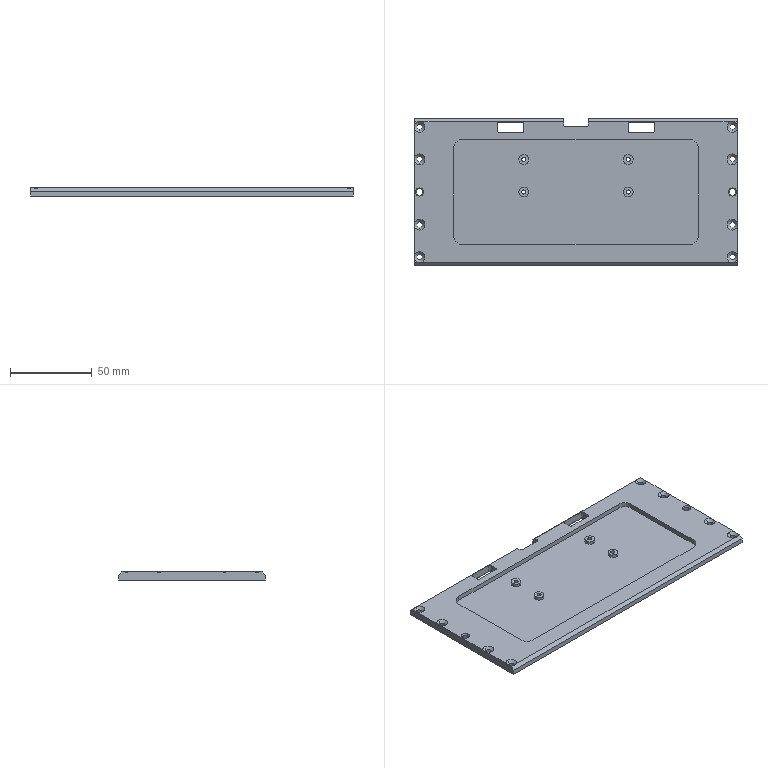NC program | NX | posted with a generic post | part box 198 x 90 x 5 mm
Lines 3800 to 4593 of 7766:
(ZLEVEL_PROFILE_COPY_1_COPY_COPY_COPY_1 , TOOL : D6A45)
N7532 T01 M6
N7534 G54
N7536 G17 G0 G90 X-98.549 Y18.596 S9500 M3
N7538 G43 Z30. H1
N7540 Z1.5
N7542 G94 G1 X-98.417 Y18.395 Z1.487 F1000.
N7544 X-98.284 Y18.195 Z1.475
N7546 X-97.848 Y17.753 Z1.442
N7548 X-97.329 Y17.413 Z1.41
N7550 X-96.75 Y17.192 Z1.377
N7552 X-96.137 Y17.098 Z1.345
N7554 X-95.518 Y17.136 Z1.312
N7556 X-94.921 Y17.304 Z1.28
N7558 X-94.373 Y17.596 Z1.247
N7560 X-93.998 Y17.898 Z1.222
N7562 X-93.598 Y18.372 Z1.189
N7564 X-93.306 Y18.92 Z1.157
N7566 X-93.138 Y19.517 Z1.124
N7568 X-93.1 Y20.136 Z1.092
N7570 X-93.194 Y20.749 Z1.059
N7572 X-93.416 Y21.328 Z1.027
N7574 X-93.756 Y21.847 Z0.994
N7576 X-93.923 Y22.02 Z0.982
N7578 X-94.092 Y22.193 Z0.969
N7580 X-94.624 Y22.56 Z0.935
N7582 X-95.224 Y22.801 Z0.901
N7584 X-95.862 Y22.903 Z0.868
N7586 X-96.507 Y22.862 Z0.834
N7588 X-97.128 Y22.681 Z0.8
N7590 X-97.692 Y22.366 Z0.766
N7592 X-98.174 Y21.936 Z0.732
N7594 X-98.32 Y21.743 Z0.719
N7596 X-98.46 Y21.586 Z0.708
N7598 X-98.679 Y21.219 Z0.686
N7600 X-98.835 Y20.79 Z0.662
N7602 X-98.933 Y20.214 Z0.631
N7604 X-98.917 Y19.63 Z0.601
N7606 X-98.79 Y19.06 Z0.57
N7608 X-98.694 Y18.834 Z0.557
N7610 X-98.679 Y18.795 Z0.555
N7612 X-98.417 Y18.395 Z0.53
N7614 X-98.284 Y18.195 Z0.517
N7616 X-97.848 Y17.753 Z0.485
N7618 X-97.329 Y17.413 Z0.452
N7620 X-96.75 Y17.192 Z0.42
N7622 X-96.137 Y17.098 Z0.387
N7624 X-95.518 Y17.136 Z0.355
N7626 X-94.921 Y17.304 Z0.322
N7628 X-94.373 Y17.596 Z0.29
N7630 X-93.998 Y17.898 Z0.265
N7632 X-93.598 Y18.372 Z0.232
N7634 X-93.306 Y18.92 Z0.2
N7636 X-93.138 Y19.517 Z0.167
N7638 X-93.1 Y20.136 Z0.135
N7640 X-93.194 Y20.749 Z0.102
N7642 X-93.416 Y21.328 Z0.07
N7644 X-93.756 Y21.847 Z0.037
N7646 X-93.923 Y22.02 Z0.024
N7648 X-94.092 Y22.193 Z0.012
N7650 X-94.624 Y22.56 Z-0.022
N7652 X-95.224 Y22.801 Z-0.056
N7654 X-95.862 Y22.903 Z-0.09
N7656 X-96.507 Y22.862 Z-0.124
N7658 X-97.128 Y22.681 Z-0.158
N7660 X-97.692 Y22.366 Z-0.191
N7662 X-98.174 Y21.936 Z-0.225
N7664 X-98.32 Y21.743 Z-0.238
N7666 X-98.46 Y21.586 Z-0.249
N7668 X-98.679 Y21.219 Z-0.271
N7670 X-98.835 Y20.79 Z-0.295
N7672 X-98.933 Y20.214 Z-0.326
N7674 X-98.917 Y19.63 Z-0.357
N7676 X-98.79 Y19.06 Z-0.387
N7678 X-98.694 Y18.834 Z-0.4
N7680 X-98.679 Y18.795 F1300.
N7682 X-98.417 Y18.395
N7684 G3 X-93.923 Y22.02 R-2.899
N7686 X-98.32 Y21.743 R2.904
N7688 X-98.751 Y21.02 R2.219
N7690 X-98.694 Y18.834 R3.
N7692 G1 X-98.678 Y18.795 Z-0.401
N7694 X-98.543 Y18.599 Z-0.407
N7696 X-98.381 Y18.366 Z-0.413
N7698 X-98.246 Y18.197 Z-0.418
N7700 X-98.099 Y18.037 Z-0.424
N7702 X-97.925 Y17.874 Z-0.429
N7704 X-97.739 Y17.726 Z-0.435
N7706 X-97.54 Y17.597 Z-0.44
N7708 X-97.334 Y17.479 Z-0.446
N7710 X-97.116 Y17.387 Z-0.452
N7712 X-96.894 Y17.304 Z-0.457
N7714 X-96.665 Y17.251 Z-0.463
N7716 X-96.435 Y17.203 Z-0.468
N7718 X-96.195 Y17.184 Z-0.474
N7720 X-95.966 Y17.182 Z-0.479
N7722 X-95.733 Y17.206 Z-0.485
N7724 X-95.502 Y17.24 Z-0.49
N7726 X-95.277 Y17.298 Z-0.496
N7728 X-95.056 Y17.372 Z-0.501
N7730 X-94.843 Y17.463 Z-0.507
N7732 X-94.739 Y17.516 Z-0.51
N7734 X-94.639 Y17.575 Z-0.512
N7736 X-94.443 Y17.697 Z-0.518
N7738 X-94.263 Y17.843 Z-0.523
N7740 X-94.165 Y17.926 Z-0.526
N7742 X-94.048 Y18.044 Z-0.53
N7744 X-93.938 Y18.168 Z-0.534
N7746 X-93.796 Y18.348 Z-0.539
N7748 X-93.67 Y18.54 Z-0.545
N7750 X-93.564 Y18.742 Z-0.55
N7752 X-93.469 Y18.95 Z-0.556
N7754 X-93.4 Y19.167 Z-0.561
N7756 X-93.337 Y19.386 Z-0.566
N7758 X-93.303 Y19.613 Z-0.572
N7760 X-93.285 Y19.836 Z-0.577
N7762 X-93.291 Y20.062 Z-0.582
N7764 X-93.309 Y20.287 Z-0.588
N7766 X-93.348 Y20.508 Z-0.593
N7768 X-93.403 Y20.726 Z-0.598
N7770 X-93.477 Y20.937 Z-0.604
N7772 X-93.568 Y21.142 Z-0.609
N7774 X-93.674 Y21.338 Z-0.614
N7776 X-93.799 Y21.524 Z-0.62
N7778 X-93.937 Y21.697 Z-0.625
N7780 X-94.088 Y21.86 Z-0.63
N7782 X-94.163 Y21.929 Z-0.632
N7784 X-94.239 Y21.997 Z-0.635
N7786 X-94.408 Y22.129 Z-0.64
N7788 X-94.585 Y22.239 Z-0.645
N7790 X-94.765 Y22.343 Z-0.65
N7792 X-94.956 Y22.423 Z-0.655
N7794 X-95.149 Y22.498 Z-0.66
N7796 X-95.35 Y22.546 Z-0.664
N7798 X-95.552 Y22.592 Z-0.669
N7800 X-95.962 Y22.621 Z-0.679
N7802 X-96.371 Y22.585 Z-0.689
N7804 X-96.768 Y22.487 Z-0.698
N7806 X-96.957 Y22.41 Z-0.703
N7808 X-97.143 Y22.329 Z-0.708
N7810 X-97.487 Y22.114 Z-0.718
N7812 X-97.791 Y21.848 Z-0.727
N7814 X-98.052 Y21.542 Z-0.737
N7816 X-98.109 Y21.46 Z-0.739
N7818 X-98.202 Y21.323 Z-0.743
N7820 X-98.327 Y21.114 Z-0.749
N7822 X-98.38 Y21.004 Z-0.752
N7824 X-98.42 Y20.889 Z-0.754
N7826 X-98.469 Y20.703 Z-0.759
N7828 X-98.516 Y20.515 Z-0.764
N7830 X-98.537 Y20.325 Z-0.768
N7832 X-98.556 Y20.133 Z-0.773
N7834 Y20.015 Z-0.775
N7836 X-98.535 Y19.734 Z-0.782
N7838 X-98.498 Y19.547 Z-0.787
N7840 X-98.46 Y19.361 Z-0.791
N7842 X-98.4 Y19.182 Z-0.796
N7844 X-98.325 Y19.009 Z-0.8
N7846 X-98.266 Y18.899 Z-0.803
N7848 X-98.199 Y18.793 Z-0.807
N7850 X-98.051 Y18.594 Z-0.814
N7852 X-97.917 Y18.432 Z-0.82
N7854 X-97.775 Y18.279 Z-0.825
N7856 X-97.616 Y18.143 Z-0.831
N7858 X-97.452 Y18.014 Z-0.837
N7860 X-97.36 Y17.954 Z-0.84
N7862 X-97.091 Y17.808 Z-0.848
N7864 X-96.879 Y17.722 Z-0.855
N7866 X-96.703 Y17.666 Z-0.86
N7868 X-96.501 Y17.626 Z-0.866
N7870 X-96.298 Y17.595 Z-0.871
N7872 X-96.152 Y17.584 Z-0.875
N7874 X-96.015 Y17.577 Z-0.879
N7876 X-95.888 Y17.591 Z-0.883
N7878 X-95.686 Y17.614 Z-0.888
N7880 X-95.486 Y17.655 Z-0.894
N7882 X-95.29 Y17.709 Z-0.9
N7884 X-95.102 Y17.786 Z-0.905
N7886 X-94.921 Y17.875 Z-0.911
N7888 X-94.747 Y17.979 Z-0.917
N7890 X-94.585 Y18.098 Z-0.922
N7892 X-94.431 Y18.227 Z-0.928
N7894 X-94.294 Y18.373 Z-0.933
N7896 X-94.161 Y18.522 Z-0.939
N7898 X-94.091 Y18.625 Z-0.942
N7900 X-94.019 Y18.742 Z-0.946
N7902 X-93.949 Y18.86 Z-0.95
N7904 X-93.869 Y19.042 Z-0.955
N7906 X-93.797 Y19.227 Z-0.961
N7908 X-93.747 Y19.417 Z-0.966
N7910 X-93.708 Y19.611 Z-0.972
N7912 X-93.689 Y19.806 Z-0.977
N7914 X-93.686 Y20.003 Z-0.983
N7916 X-93.701 Y20.198 Z-0.988
N7918 X-93.73 Y20.392 Z-0.994
N7920 X-93.78 Y20.579 Z-0.999
N7922 X-93.838 Y20.765 Z-1.004
N7924 X-93.922 Y20.952 Z-1.01
N7926 X-94.007 Y21.114 Z-1.015
N7928 X-94.231 Y21.427 Z-1.026
N7930 X-94.367 Y21.562 Z-1.031
N7932 X-94.503 Y21.697 Z-1.037
N7934 X-94.605 Y21.775 Z-1.04
N7936 X-94.71 Y21.846 Z-1.044
N7938 X-94.817 Y21.915 Z-1.047
N7940 X-94.986 Y22. Z-1.052
N7942 X-95.16 Y22.076 Z-1.058
N7944 X-95.34 Y22.134 Z-1.063
N7946 X-95.524 Y22.178 Z-1.068
N7948 X-95.71 Y22.202 Z-1.073
N7950 X-95.897 Y22.217 Z-1.079
N7952 X-96.104 Y22.21 Z-1.084
N7954 X-96.27 Y22.194 Z-1.089
N7956 X-96.632 Y22.107 Z-1.099
N7958 X-96.804 Y22.039 Z-1.105
N7960 X-96.973 Y21.961 Z-1.11
N7962 X-97.128 Y21.862 Z-1.115
N7964 X-97.282 Y21.761 Z-1.12
N7966 X-97.419 Y21.639 Z-1.125
N7968 X-97.552 Y21.512 Z-1.13
N7970 X-97.644 Y21.406 Z-1.134
N7972 X-97.72 Y21.312 Z-1.137
N7974 X-97.789 Y21.214 Z-1.141
N7976 X-97.887 Y21.062 Z-1.146
N7978 X-97.985 Y20.91 Z-1.151
N7980 X-98.015 Y20.853 Z-1.153
N7982 X-98.026 Y20.822
N7984 X-98.042 Y20.767 Z-1.155
N7986 X-98.072 Y20.655 Z-1.158
N7988 X-98.107 Y20.496 Z-1.163
N7990 X-98.135 Y20.335 Z-1.167
N7992 X-98.148 Y20.174 Z-1.172
N7994 X-98.152 Y20.012 Z-1.176
N7996 X-98.142 Y19.864 Z-1.18
N7998 X-98.126 Y19.717 Z-1.184
N8000 X-98.063 Y19.429 Z-1.193
N8002 X-98.03 Y19.322 Z-1.196
N8004 X-97.999 Y19.252 Z-1.198
N8006 X-97.963 Y19.183 Z-1.2
N8008 X-97.931 Y19.11 Z-1.203
N8010 X-97.885 Y19.044 Z-1.205
N8012 X-97.73 Y18.829 Z-1.214
N8014 X-97.671 Y18.753 Z-1.217
N8016 X-97.457 Y18.533 Z-1.228
N8018 X-97.341 Y18.431 Z-1.233
N8020 X-97.234 Y18.351 Z-1.237
N8022 X-97.138 Y18.289 Z-1.241
N8024 X-96.982 Y18.207 Z-1.247
N8026 X-96.821 Y18.132 Z-1.253
N8028 X-96.785 Y18.119 Z-1.254
N8030 X-96.601 Y18.055 Z-1.261
N8032 X-96.409 Y18.016 Z-1.267
N8034 X-96.244 Y17.989 Z-1.273
N8036 X-96.115 Y17.984 Z-1.277
N8038 X-96.023 Z-1.28
N8040 X-95.832 Y18.003 Z-1.287
N8042 X-95.641 Y18.032 Z-1.293
N8044 X-95.507 Y18.063 Z-1.298
N8046 X-95.441 Y18.08 Z-1.3
N8048 X-95.385 Y18.099 Z-1.302
N8050 X-95.278 Y18.149 Z-1.306
N8052 X-95.107 Y18.231 Z-1.313
N8054 X-94.945 Y18.33 Z-1.319
N8056 X-94.821 Y18.418 Z-1.324
N8058 X-94.725 Y18.5 Z-1.328
N8060 X-94.653 Y18.569 Z-1.332
N8062 X-94.531 Y18.711 Z-1.338
N8064 X-94.417 Y18.86 Z-1.344
N8066 X-94.347 Y18.976 Z-1.349
N8068 X-94.282 Y19.095 Z-1.353
N8070 X-94.24 Y19.187 Z-1.357
N8072 X-94.179 Y19.361 Z-1.363
N8074 X-94.129 Y19.539 Z-1.369
N8076 X-94.106 Y19.67 Z-1.374
N8078 X-94.091 Y19.792 Z-1.378
N8080 X-94.087 Y19.904 Z-1.381
N8082 X-94.096 Y20.086 Z-1.388
N8084 X-94.116 Y20.267 Z-1.394
N8086 X-94.14 Y20.396 Z-1.398
N8088 X-94.158 Y20.459 Z-1.4
N8090 X-94.212 Y20.617 Z-1.406
N8092 X-94.301 Y20.812 Z-1.413
N8094 X-94.371 Y20.939 Z-1.418
N8096 X-94.488 Y21.104 Z-1.425
N8098 X-94.588 Y21.224 Z-1.43
N8100 X-94.718 Y21.345 Z-1.436
N8102 X-94.854 Y21.459 Z-1.442
N8104 X-95.023 Y21.57 Z-1.449
N8106 X-95.157 Y21.642 Z-1.454
N8108 X-95.349 Y21.716 Z-1.461
N8110 X-95.487 Y21.761 Z-1.466
N8112 X-95.664 Y21.795 Z-1.472
N8114 X-95.832 Y21.812 Z-1.478
N8116 X-95.962 Y21.817 Z-1.482
N8118 X-96.028 Y21.815 Z-1.484
N8120 X-96.178 Y21.8 Z-1.489
N8122 X-96.394 Y21.756 Z-1.497
N8124 X-96.514 Y21.725 Z-1.501
N8126 X-96.678 Y21.656 Z-1.507
N8128 X-96.826 Y21.584 Z-1.512
N8130 X-96.98 Y21.487 Z-1.518
N8132 X-97.023 Y21.456 Z-1.52
N8134 X-97.104 Y21.388 Z-1.524
N8136 X-97.225 Y21.269 Z-1.53
N8138 X-97.34 Y21.146 Z-1.535
N8140 X-97.418 Y21.048 Z-1.539
N8142 X-97.514 Y20.911 Z-1.545
N8144 X-97.572 Y20.823 Z-1.549
N8146 X-97.622 Y20.735 Z-1.552
N8148 X-97.662 Y20.65 Z-1.555
N8150 X-97.692 Y20.544 Z-1.559
N8152 X-97.717 Y20.419 Z-1.563
N8154 X-97.74 Y20.256 Z-1.569
N8156 X-97.756 Y20.093 Z-1.574
N8158 X-97.75 Y19.922 Z-1.58
N8160 X-97.732 Y19.767 Z-1.585
N8162 X-97.694 Y19.61 Z-1.59
N8164 X-97.649 Y19.454 Z-1.596
N8166 X-97.627 Y19.396 Z-1.598
N8168 X-97.597 Y19.341 Z-1.6
N8170 X-97.574 Y19.288 Z-1.602
N8172 X-97.544 Y19.239 Z-1.605
N8174 X-97.45 Y19.121 Z-1.611
N8176 X-97.327 Y18.968 Z-1.62
N8178 X-97.152 Y18.795 Z-1.63
N8180 X-97.032 Y18.701 Z-1.637
N8182 X-96.918 Y18.625 Z-1.642
N8184 X-96.815 Y18.567 Z-1.647
N8186 X-96.73 Y18.522 Z-1.652
N8188 X-96.66 Y18.497 Z-1.655
N8190 X-96.494 Y18.444 Z-1.662
N8192 X-96.323 Y18.407 Z-1.67
N8194 X-96.19 Y18.389 Z-1.675
N8196 X-96.074 Y18.385 Z-1.68
N8198 X-95.977 Y18.389 Z-1.684
N8200 X-95.835 Y18.402 Z-1.69
N8202 X-95.765 Y18.411 Z-1.693
N8204 X-95.722 Y18.421 Z-1.695
N8206 X-95.639 Y18.447 Z-1.699
N8208 X-95.478 Y18.502 Z-1.706
N8210 X-95.322 Y18.571 Z-1.714
N8212 X-95.221 Y18.628 Z-1.719
N8214 X-95.126 Y18.689 Z-1.723
N8216 X-95.043 Y18.761 Z-1.728
N8218 X-94.921 Y18.875 Z-1.735
N8220 X-94.812 Y19.002 Z-1.742
N8222 X-94.721 Y19.14 Z-1.749
N8224 X-94.64 Y19.285 Z-1.757
N8226 X-94.623 Y19.321 Z-1.758
N8228 X-94.571 Y19.455 Z-1.764
N8230 X-94.532 Y19.594 Z-1.771
N8232 X-94.505 Y19.719 Z-1.776
N8234 X-94.494 Y19.826 Z-1.781
N8236 X-94.492 Y19.916 Z-1.785
N8238 X-94.494 Y20.058 Z-1.791
N8240 X-94.5 Y20.128 Z-1.794
N8242 X-94.507 Y20.165 Z-1.795
N8244 X-94.521 Y20.237 Z-1.798
N8246 X-94.555 Y20.375 Z-1.804
N8248 X-94.59 Y20.475 Z-1.809
N8250 X-94.618 Y20.541 Z-1.812
N8252 X-94.676 Y20.657 Z-1.818
N8254 X-94.706 Y20.714 Z-1.82
N8256 X-94.727 Y20.749 Z-1.822
N8258 X-94.775 Y20.815 Z-1.826
N8260 X-94.862 Y20.927 Z-1.832
N8262 X-94.936 Y21. Z-1.836
N8264 X-94.984 Y21.048 Z-1.839
N8266 X-95.077 Y21.121 Z-1.844
N8268 X-95.16 Y21.182 Z-1.848
N8270 X-95.237 Y21.228 Z-1.852
N8272 X-95.348 Y21.285 Z-1.858
N8274 X-95.406 Y21.309 Z-1.86
N8276 X-95.518 Y21.349 Z-1.865
N8278 X-95.667 Y21.38 Z-1.872
N8280 X-95.816 Y21.409 Z-1.879
N8282 X-95.991 Y21.414 Z-1.886
N8284 X-96.108 Y21.401 Z-1.891
N8286 X-96.238 Y21.381 Z-1.897
N8288 X-96.336 Y21.354 Z-1.901
N8290 X-96.404 Y21.332 Z-1.904
N8292 X-96.514 Y21.288 Z-1.909
N8294 X-96.606 Y21.247 Z-1.913
N8296 X-96.675 Y21.198 Z-1.917
N8298 X-96.798 Y21.113 Z-1.923
N8300 X-96.914 Y21.018 Z-1.93
N8302 X-97.11 Y20.794 Z-1.943
N8304 X-97.184 Y20.682 Z-1.948
N8306 X-97.207 Y20.646 Z-1.95
N8308 X-97.259 Y20.564 Z-1.954
N8310 X-97.288 Y20.506 Z-1.957
N8312 X-97.309 Y20.414 Z-1.961
N8314 X-97.331 Y20.296 Z-1.966
N8316 X-97.351 Y20.177 Z-1.971
N8318 X-97.356 Y20.054 Z-1.977
N8320 X-97.352 Y19.939 Z-1.982
N8322 X-97.312 Y19.706 Z-1.992
N8324 X-97.251 Y19.52 Z-2.
N8326 X-97.027 Y19.21
N8328 G3 X-95.992 Y21.299 R-1.297
N8330 X-97.219 Y20.546 R1.491
N8332 X-97.251 Y19.52 R1.389
N8334 G1 Z-0.5
N8336 G0 Z30.
N8338 X-98.49 Y38.508
N8340 Z1.5
N8342 G1 X-98.419 Y38.399 Z1.493 F1000.
N8344 X-98.286 Y38.198 Z1.481
N8346 X-97.842 Y37.746 Z1.447
N8348 X-97.312 Y37.401 Z1.414
N8350 X-96.719 Y37.179 Z1.381
N8352 X-96.091 Y37.09 Z1.348
N8354 X-95.46 Y37.139 Z1.315
N8356 X-94.854 Y37.324 Z1.281
N8358 X-94.303 Y37.635 Z1.248
N8360 X-93.936 Y37.947 Z1.223
N8362 X-93.541 Y38.443 Z1.19
N8364 X-93.263 Y39.012 Z1.157
N8366 X-93.114 Y39.627 Z1.123
N8368 X-93.102 Y40.26 Z1.09
N8370 X-93.227 Y40.881 Z1.057
N8372 X-93.484 Y41.46 Z1.024
N8374 X-93.86 Y41.97 Z0.991
N8376 X-94.037 Y42.133 Z0.978
N8378 X-94.208 Y42.299 Z0.965
N8380 X-94.696 Y42.622 Z0.935
N8382 X-95.24 Y42.837 Z0.904
N8384 X-95.816 Y42.938 Z0.874
N8386 X-96.401 Y42.918 Z0.843
N8388 X-96.969 Y42.779 Z0.812
N8390 X-97.186 Y42.68 Z0.8
N8392 X-97.453 Y42.519 Z0.783
N8394 X-97.679 Y42.374 Z0.769
N8396 X-98.046 Y42.057 Z0.744
N8398 X-98.368 Y41.694 Z0.718
N8400 X-98.516 Y41.47 Z0.704
N8402 X-98.644 Y41.276 Z0.692
N8404 X-98.655 Y41.254 Z0.691
N8406 X-98.758 Y41.031 Z0.678
N8408 X-98.916 Y40.382 Z0.643
N8410 X-98.927 Y39.714 Z0.608
N8412 X-98.792 Y39.059 Z0.573
N8414 X-98.691 Y38.817 Z0.559
N8416 X-98.419 Y38.399 Z0.533
N8418 X-98.286 Y38.198 Z0.52
N8420 X-97.842 Y37.746 Z0.487
N8422 X-97.312 Y37.401 Z0.454
N8424 X-96.719 Y37.179 Z0.421
N8426 X-96.091 Y37.09 Z0.388
N8428 X-95.46 Y37.139 Z0.355
N8430 X-94.854 Y37.324 Z0.321
N8432 X-94.303 Y37.635 Z0.288
N8434 X-93.936 Y37.947 Z0.263
N8436 X-93.541 Y38.443 Z0.23
N8438 X-93.263 Y39.012 Z0.196
N8440 X-93.114 Y39.627 Z0.163
N8442 X-93.102 Y40.26 Z0.13
N8444 X-93.227 Y40.881 Z0.097
N8446 X-93.484 Y41.46 Z0.064
N8448 X-93.86 Y41.97 Z0.031
N8450 X-94.037 Y42.133 Z0.018
N8452 X-94.208 Y42.299 Z0.005
N8454 X-94.696 Y42.622 Z-0.025
N8456 X-95.24 Y42.837 Z-0.056
N8458 X-95.816 Y42.938 Z-0.087
N8460 X-96.401 Y42.918 Z-0.117
N8462 X-96.969 Y42.779 Z-0.148
N8464 X-97.186 Y42.68 Z-0.16
N8466 X-97.453 Y42.519 Z-0.177
N8468 X-97.679 Y42.374 Z-0.191
N8470 X-98.046 Y42.057 Z-0.216
N8472 X-98.368 Y41.694 Z-0.242
N8474 X-98.516 Y41.47 Z-0.256
N8476 X-98.644 Y41.276 Z-0.268
N8478 X-98.655 Y41.254 Z-0.269
N8480 X-98.758 Y41.031 Z-0.282
N8482 X-98.916 Y40.382 Z-0.317
N8484 X-98.927 Y39.714 Z-0.352
N8486 X-98.792 Y39.059 Z-0.387
N8488 X-98.698 Y38.832 Z-0.4
N8490 X-98.691 Y38.817 F1300.
N8492 X-98.419 Y38.399
N8494 G3 X-94.037 Y42.133 R-2.9
N8496 X-97.186 Y42.68 R2.836
N8498 G1 X-97.453 Y42.519
N8500 G3 X-98.516 Y41.47 R3.61
N8502 G1 X-98.644 Y41.276
N8504 X-98.655 Y41.254
N8506 G3 X-98.698 Y38.832 R3.02
N8508 G1 X-98.556 Y38.618 Z-0.406
N8510 X-98.409 Y38.406 Z-0.412
N8512 X-98.275 Y38.229 Z-0.417
N8514 X-98.128 Y38.063 Z-0.423
N8516 X-97.97 Y37.909 Z-0.428
N8518 X-97.799 Y37.768 Z-0.433
N8520 X-97.568 Y37.606 Z-0.44
N8522 X-97.432 Y37.528 Z-0.443
N8524 X-97.236 Y37.428 Z-0.448
N8526 X-97.032 Y37.347 Z-0.454
N8528 X-96.825 Y37.28 Z-0.459
N8530 X-96.612 Y37.23 Z-0.464
N8532 X-96.397 Y37.197 Z-0.469
N8534 X-96.18 Y37.179 Z-0.474
N8536 X-95.963 Y37.18 Z-0.479
N8538 X-95.746 Y37.195 Z-0.484
N8540 X-95.533 Y37.23 Z-0.49
N8542 X-95.322 Y37.277 Z-0.495
N8544 X-95.118 Y37.344 Z-0.5
N8546 X-94.917 Y37.423 Z-0.505
N8548 X-94.726 Y37.52 Z-0.51
N8550 X-94.541 Y37.628 Z-0.515
N8552 X-94.368 Y37.753 Z-0.52
N8554 X-94.201 Y37.887 Z-0.525
N8556 X-94.05 Y38.037 Z-0.53
N8558 X-93.906 Y38.195 Z-0.535
N8560 X-93.846 Y38.266 Z-0.537
N8562 X-93.663 Y38.542 Z-0.545
N8564 X-93.566 Y38.73 Z-0.55
N8566 X-93.477 Y38.921 Z-0.555
N8568 X-93.41 Y39.121 Z-0.56
N8570 X-93.351 Y39.323 Z-0.565
N8572 X-93.316 Y39.53 Z-0.57
N8574 X-93.288 Y39.738 Z-0.575
N8576 X-93.285 Y39.947 Z-0.58
N8578 X-93.289 Y40.156 Z-0.585
N8580 X-93.32 Y40.362 Z-0.59
N8582 X-93.355 Y40.568 Z-0.595
N8584 X-93.417 Y40.766 Z-0.599
N8586 X-93.481 Y40.963 Z-0.604
N8588 X-93.573 Y41.149 Z-0.609
N8590 X-93.667 Y41.334 Z-0.614
N8592 X-93.906 Y41.67 Z-0.624
N8594 X-94.133 Y41.907 Z-0.632
N8596 X-94.198 Y41.969 Z-0.634
N8598 X-94.505 Y42.206 Z-0.643
N8600 X-94.834 Y42.407 Z-0.652
N8602 X-94.93 Y42.457 Z-0.654
N8604 X-94.98 Y42.477 Z-0.656
N8606 X-95.051 Y42.5 Z-0.657
N8608 X-95.195 Y42.543 Z-0.661
N8610 X-95.339 Y42.579 Z-0.665
N8612 X-95.485 Y42.609 Z-0.668
N8614 X-95.574 Y42.624 Z-0.67
N8616 X-95.764 Y42.641 Z-0.675
N8618 X-95.955 Y42.651 Z-0.679
N8620 X-96.145 Y42.638 Z-0.684
N8622 X-96.335 Y42.622 Z-0.688
N8624 X-96.52 Y42.582 Z-0.693
N8626 X-96.704 Y42.536 Z-0.697
N8628 X-96.855 Y42.489 Z-0.701
N8630 X-96.929 Y42.462 Z-0.703
N8632 X-96.973 Y42.444 Z-0.704
N8634 X-97.058 Y42.401 Z-0.706
N8636 X-97.292 Y42.253 Z-0.713
N8638 X-97.472 Y42.121 Z-0.718
N8640 X-97.647 Y41.983 Z-0.723
N8642 X-97.72 Y41.914 Z-0.725
N8644 X-97.792 Y41.844 Z-0.728
N8646 X-97.961 Y41.653 Z-0.734
N8648 X-98.098 Y41.466 Z-0.739
N8650 X-98.233 Y41.277 Z-0.745
N8652 X-98.33 Y41.119 Z-0.749
N8654 X-98.377 Y41.026 Z-0.752
N8656 X-98.395 Y40.977 Z-0.753
N8658 X-98.417 Y40.906 Z-0.755
N8660 X-98.458 Y40.762 Z-0.758
N8662 X-98.5 Y40.584 Z-0.762
N8664 X-98.531 Y40.404 Z-0.767
N8666 X-98.545 Y40.223 Z-0.771
N8668 X-98.554 Y40.041 Z-0.775
N8670 X-98.543 Y39.86 Z-0.78
N8672 X-98.527 Y39.679 Z-0.784
N8674 X-98.45 Y39.326 Z-0.792
N8676 X-98.397 Y39.174 Z-0.796
N8678 X-98.341 Y39.019 Z-0.8
N8680 X-98.198 Y38.79 Z-0.807
N8682 X-98.131 Y38.699 Z-0.811
N8684 X-98.064 Y38.608 Z-0.814
N8686 X-97.907 Y38.418 Z-0.82
N8688 X-97.735 Y38.242 Z-0.827
N8690 X-97.679 Y38.187 Z-0.829
N8692 X-97.617 Y38.138 Z-0.832
N8694 X-97.483 Y38.039 Z-0.836
N8696 X-97.349 Y37.941 Z-0.841
N8698 X-97.173 Y37.845 Z-0.846
N8700 X-96.991 Y37.76 Z-0.852
N8702 X-96.802 Y37.697 Z-0.857
N8704 X-96.61 Y37.64 Z-0.863
N8706 X-96.414 Y37.606 Z-0.868
N8708 X-96.217 Y37.584 Z-0.874
N8710 X-96.019 Y37.58 Z-0.879
N8712 X-95.821 Y37.592 Z-0.885
N8714 X-95.626 Y37.62 Z-0.89
N8716 X-95.434 Y37.665 Z-0.896
N8718 X-95.247 Y37.725 Z-0.901
N8720 X-95.065 Y37.799 Z-0.907
N8722 X-94.892 Y37.889 Z-0.912
N8724 X-94.724 Y37.99 Z-0.917
N8726 X-94.57 Y38.107 Z-0.923
N8728 X-94.42 Y38.232 Z-0.928
N8730 X-94.288 Y38.374 Z-0.933
N8732 X-94.16 Y38.519 Z-0.939
N8734 X-94.049 Y38.682 Z-0.944
N8736 X-93.953 Y38.844 Z-0.949
N8738 X-93.875 Y39.02 Z-0.955
N8740 X-93.804 Y39.198 Z-0.96
N8742 X-93.753 Y39.382 Z-0.965
N8744 X-93.713 Y39.569 Z-0.971
N8746 X-93.692 Y39.758 Z-0.976
N8748 X-93.684 Y39.948 Z-0.981
N8750 X-93.692 Y40.137 Z-0.986
N8752 X-93.716 Y40.325 Z-0.992
N8754 X-93.754 Y40.509 Z-0.997
N8756 X-93.81 Y40.69 Z-1.002
N8758 X-93.878 Y40.864 Z-1.007
N8760 X-93.96 Y41.033 Z-1.012
N8762 X-94.035 Y41.161 Z-1.017
N8764 X-94.119 Y41.284 Z-1.021
N8766 X-94.165 Y41.347 Z-1.023
N8768 X-94.289 Y41.487 Z-1.028
N8770 X-94.415 Y41.624 Z-1.033
N8772 X-94.675 Y41.831 Z-1.042
N8774 X-94.951 Y42.012 Z-1.052
N8776 X-95.046 Y42.069 Z-1.055
N8778 X-95.096 Y42.092 Z-1.056
N8780 X-95.147 Y42.111 Z-1.058
N8782 X-95.253 Y42.143 Z-1.061
N8784 X-95.408 Y42.183 Z-1.065
N8786 X-95.564 Y42.218 Z-1.069
N8788 X-95.744 Y42.237 Z-1.075
N8790 X-95.925 Y42.251 Z-1.08
N8792 X-96.104 Y42.239 Z-1.084
N8794 X-96.284 Y42.224 Z-1.089
N8796 X-96.459 Y42.185 Z-1.094
N8798 X-96.633 Y42.141 Z-1.099
N8800 X-96.768 Y42.089 Z-1.103
N8802 X-96.901 Y42.033 Z-1.107
N8804 X-96.939 Y42.011 Z-1.109
N8806 X-97.24 Y41.801 Z-1.119
N8808 X-97.376 Y41.679 Z-1.124
N8810 X-97.512 Y41.556 Z-1.129
N8812 X-97.642 Y41.406 Z-1.134
N8814 X-97.767 Y41.25 Z-1.14
N8816 X-97.911 Y41.034 Z-1.147
N8818 X-97.967 Y40.941 Z-1.15
N8820 X-98.02 Y40.84 Z-1.153
N8822 X-98.056 Y40.724 Z-1.157
N8824 X-98.089 Y40.597 Z-1.16
N8826 X-98.122 Y40.418 Z-1.165
N8828 X-98.149 Y40.238 Z-1.17
N8830 X-98.155 Y40.046 Z-1.175
N8832 X-98.148 Y39.877 Z-1.18
N8834 X-98.121 Y39.699 Z-1.185
N8836 X-98.085 Y39.523 Z-1.19
N8838 X-98.027 Y39.31 Z-1.196
N8840 X-97.979 Y39.182 Z-1.2
N8842 X-97.96 Y39.186
N8844 X-97.931 Y39.109 Z-1.203
N8846 X-97.885 Y39.042 Z-1.205
N8848 X-97.791 Y38.908 Z-1.211
N8850 X-97.705 Y38.793 Z-1.216
N8852 X-97.589 Y38.655 Z-1.222
N8854 X-97.471 Y38.546 Z-1.227
N8856 X-97.351 Y38.438 Z-1.232
N8858 X-97.243 Y38.354 Z-1.237
N8860 X-97.189 Y38.313 Z-1.239
N8862 X-97.142 Y38.283 Z-1.241
N8864 X-97.043 Y38.231 Z-1.245
N8866 X-96.878 Y38.15 Z-1.251
N8868 X-96.705 Y38.084 Z-1.257
N8870 X-96.528 Y38.037 Z-1.263
N8872 X-96.348 Y38. Z-1.269
N8874 X-96.145 Y37.982 Z-1.276
N8876 X-95.984 Y37.981 Z-1.282
N8878 X-95.853 Y37.992 Z-1.286
N8880 X-95.732 Y38.005 Z-1.29
N8882 X-95.625 Y38.03 Z-1.294
N8884 X-95.452 Y38.079 Z-1.3
N8886 X-95.282 Y38.14 Z-1.306
N8888 X-95.121 Y38.218 Z-1.312
N8890 X-94.967 Y38.309 Z-1.318
N8892 X-94.877 Y38.373 Z-1.321
N8894 X-94.762 Y38.463 Z-1.326
N8896 X-94.697 Y38.523 Z-1.329
N8898 X-94.569 Y38.662 Z-1.336
N8900 X-94.448 Y38.807 Z-1.342
N8902 X-94.404 Y38.87 Z-1.345
N8904 X-94.339 Y38.983 Z-1.349
N8906 X-94.275 Y39.097 Z-1.353
N8908 X-94.224 Y39.214 Z-1.358
N8910 X-94.198 Y39.272 Z-1.36
N8912 X-94.181 Y39.322 Z-1.361
N8914 X-94.152 Y39.424 Z-1.365
N8916 X-94.116 Y39.594 Z-1.371
N8918 X-94.091 Y39.766 Z-1.377
N8920 X-94.084 Y39.958 Z-1.383
N8922 X-94.091 Y40.111 Z-1.388
N8924 X-94.121 Y40.308 Z-1.395
N8926 X-94.153 Y40.449 Z-1.4
N8928 X-94.193 Y40.571 Z-1.404
N8930 X-94.23 Y40.678 Z-1.408
N8932 X-94.275 Y40.767 Z-1.411
N8934 X-94.357 Y40.916 Z-1.417
N8936 X-94.45 Y41.058 Z-1.423
N8938 X-94.544 Y41.175 Z-1.428
N8940 X-94.646 Y41.286 Z-1.433
N8942 X-94.749 Y41.378 Z-1.437
N8944 X-94.883 Y41.488 Z-1.443
N8946 X-95.006 Y41.569 Z-1.448
N8948 X-95.129 Y41.649 Z-1.453
N8950 X-95.223 Y41.705 Z-1.457
N8952 X-95.272 Y41.731 Z-1.458
N8954 X-95.312 Y41.745 Z-1.46
N8956 X-95.397 Y41.767 Z-1.463
N8958 X-95.564 Y41.809 Z-1.469
N8960 X-95.733 Y41.842 Z-1.474
N8962 X-95.906 Y41.85 Z-1.48
N8964 X-96.076 Y41.847 Z-1.486
N8966 X-96.265 Y41.822 Z-1.492
N8968 X-96.411 Y41.79 Z-1.497
N8970 X-96.549 Y41.749 Z-1.502
N8972 X-96.654 Y41.709 Z-1.506
N8974 X-96.727 Y41.672 Z-1.509
N8976 X-96.843 Y41.591 Z-1.513
N8978 X-96.984 Y41.492 Z-1.519
N8980 X-97.229 Y41.275 Z-1.53
N8982 X-97.334 Y41.15 Z-1.535
N8984 X-97.437 Y41.023 Z-1.541
N8986 X-97.551 Y40.849 Z-1.548
N8988 X-97.604 Y40.767 Z-1.551
N8990 X-97.651 Y40.684 Z-1.554
N8992 X-97.679 Y40.589 Z-1.558
N8994 X-97.706 Y40.49 Z-1.561
N8996 X-97.729 Y40.344 Z-1.566
N8998 X-97.751 Y40.199 Z-1.571
N9000 X-97.756 Y40.049 Z-1.576
N9002 X-97.751 Y39.907 Z-1.581
N9004 X-97.726 Y39.732 Z-1.587
N9006 X-97.703 Y39.62 Z-1.59
N9008 X-97.657 Y39.483 Z-1.595
N9010 X-97.599 Y39.351 Z-1.6
N9012 X-97.558 Y39.263 Z-1.604
N9014 X-97.501 Y39.185 Z-1.608
N9016 X-97.386 Y39.032 Z-1.616
N9018 X-97.322 Y38.955 Z-1.62
N9020 X-97.151 Y38.785 Z-1.631
N9022 X-97.006 Y38.677 Z-1.638
N9024 X-96.876 Y38.592 Z-1.645
N9026 X-96.715 Y38.511 Z-1.652
N9028 X-96.569 Y38.46 Z-1.659
N9030 X-96.434 Y38.422 Z-1.665
N9032 X-96.326 Y38.402 Z-1.669
N9034 X-96.246 Y38.389 Z-1.673
N9036 X-96.124 Y38.383 Z-1.678
N9038 X-96.015 Y38.379 Z-1.683
N9040 X-95.917 Y38.389 Z-1.687
N9042 X-95.756 Y38.412 Z-1.694
N9044 X-95.598 Y38.453 Z-1.701
N9046 X-95.472 Y38.494 Z-1.706
N9048 X-95.374 Y38.538 Z-1.711
N9050 X-95.299 Y38.576 Z-1.714
N9052 X-95.165 Y38.663 Z-1.721
N9054 X-95.036 Y38.758 Z-1.728
N9056 X-94.92 Y38.867 Z-1.735
N9058 X-94.844 Y38.95 Z-1.739
N9060 X-94.779 Y39.027 Z-1.744
N9062 X-94.733 Y39.103 Z-1.747
N9064 X-94.658 Y39.23 Z-1.754
N9066 X-94.596 Y39.365 Z-1.76
N9068 X-94.541 Y39.525 Z-1.767
N9070 X-94.512 Y39.645 Z-1.772
N9072 X-94.49 Y39.81 Z-1.779
N9074 X-94.484 Y39.934 Z-1.785
N9076 X-94.488 Y40.046 Z-1.789
N9078 X-94.49 Y40.102 Z-1.792
N9080 X-94.497 Y40.142 Z-1.793
N9082 X-94.511 Y40.221 Z-1.797
N9084 X-94.548 Y40.359 Z-1.803
N9086 X-94.591 Y40.496 Z-1.809
N9088 X-94.655 Y40.631 Z-1.815
N9090 X-94.72 Y40.748 Z-1.821
N9092 X-94.894 Y40.97 Z-1.833
N9094 X-95.017 Y41.085 Z-1.84
N9096 X-95.111 Y41.16 Z-1.845
N9098 X-95.281 Y41.274 Z-1.854
N9100 X-95.363 Y41.32 Z-1.858
N9102 X-95.462 Y41.373 Z-1.863
N9104 X-95.556 Y41.401 Z-1.867
N9106 X-95.641 Y41.419 Z-1.871
N9108 X-95.786 Y41.438 Z-1.877
N9110 X-95.932 Y41.452 Z-1.883
N9112 X-96.07 Y41.444 Z-1.889